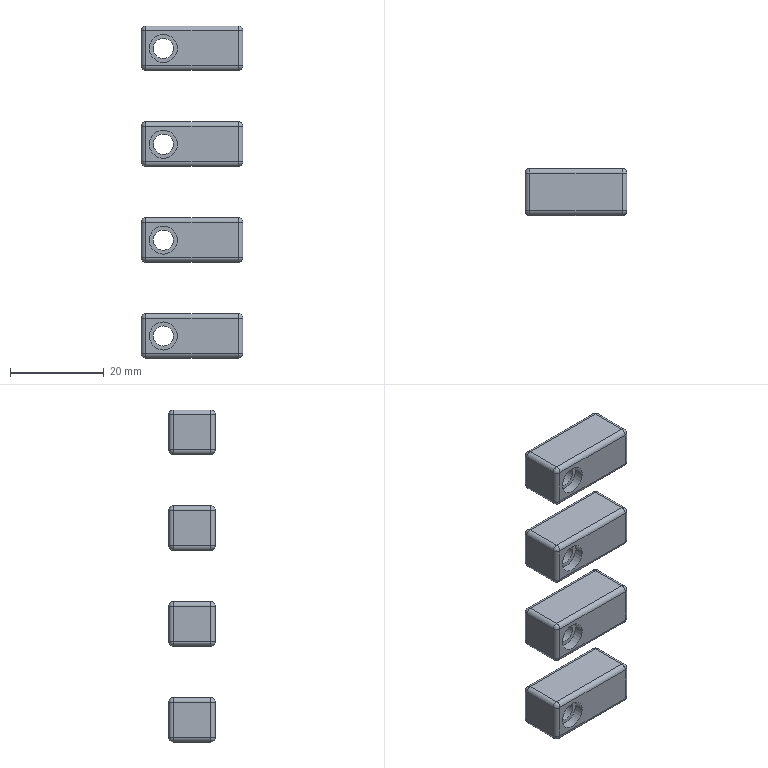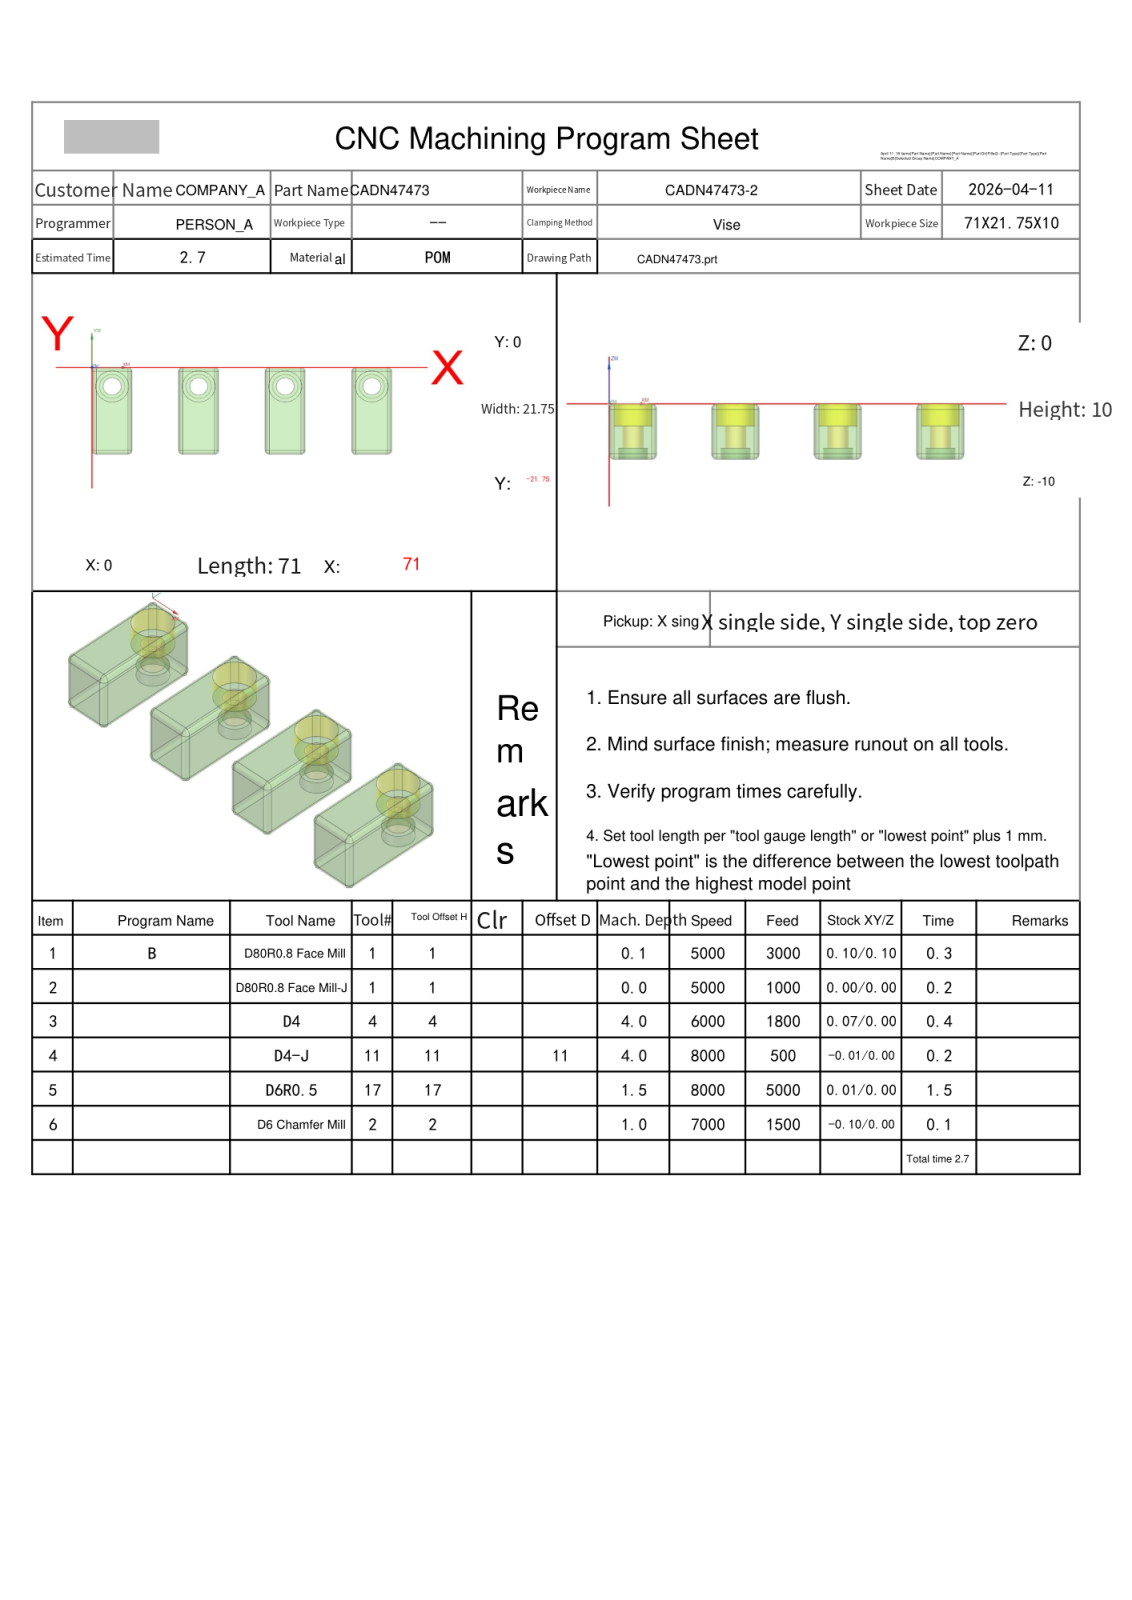NC program | NX | posted by the shop | part box 21.75 x 10 x 71 mm
Lines 1 to 259 of 15118:
%
O0001
(Machine time: 3.82 MIN)
(===Total Tool:5===)
(T1=D80R0.8 Face Mill D=80.  R=0.8  D-  H01 Z=0.    )
(T4=D4      D=4.   R=0.   D-  H04 Z=-4.   )
(T11=D4-J   D=4.   R=0.   D11 H11 Z=-4.   )
(T17=D6R0.5 D=6.   R=0.5  D-  H17 Z=-1.5  )
(T2=D6 Chamfer Mill   D=6.   R=0.   D-  H02 Z=-1.   )
G80 G90 G17 G49 G40
G91 G28 Z0
M01
N1 T01 M06
(D80R0.8 Face Mill  D=80. R=0.8 H=01 ce=0.10 di=0.10)
G00 G90 G54 X-52.097 Y-10.875 M03 S5000
G43 H01 Z20.
M08
Z3.525
G01 Z1.525 F3000.
X-40.097
X111.097
X123.097
Z3.525
G00 X-52.097
Z3.05
G01 Z1.05
X-40.097
X111.097
X123.097
Z3.05
G00 X-52.097
Z2.575
G01 Z.575
X-40.097
X111.097
X123.097
Z2.575
G00 X-52.097
Z2.1
G01 Z.1
X-40.097
X111.097
X123.097
Z2.1
G00 Z20.
G91 G28 Z0.0
M05
M09
G91 G28 Z0.0
M01
N2 T01 M06
(D80R0.8 Face Mill-J  D=80. R=0.8 H=01 ce=0.00 di=0.00)
G00 G90 G54 X-51.999 Y-10.875 M03 S5000
G43 H01 Z20.
M08
Z2.
G01 Z0.0 F1000.
X-39.999
X110.999
X122.999
Z2.
G00 Z20.
G91 G28 Z0.0
M05
M09
G91 G28 Z0.0
M01
N3 T04 M06
(D4  D=4. R=0. H=04 ce=0.07 di=0.00)
G00 G90 G54 X66.296 Y-4.75 M03 S6000
G43 H04 Z20.
M08
Z.3
G03 X65.381 Y-5.665 I0.0 J-.915 F1800.
X66.296 Y-6.58 I.915 J0.0
X66.296 Y-6.58 Z-.05 I0.0 J1.83
X66.296 Y-6.58 Z-.4 I0.0 J1.83
X66.296 Y-6.58 Z-.75 I0.0 J1.83
X66.296 Y-6.58 Z-1.1 I0.0 J1.83
X66.296 Y-6.58 Z-1.45 I0.0 J1.83
X66.296 Y-6.58 Z-1.8 I0.0 J1.83
X66.296 Y-6.58 Z-2.15 I0.0 J1.83
X66.296 Y-6.58 Z-2.5 I0.0 J1.83
X66.296 Y-6.58 Z-2.85 I0.0 J1.83
X66.296 Y-6.58 Z-3.2 I0.0 J1.83
X66.296 Y-6.58 Z-3.55 I0.0 J1.83
X66.296 Y-6.58 Z-3.9 I0.0 J1.83
X68.08 Y-4.343 Z-4. I0.0 J1.83
X66.296 Y-2.92 I-1.784 J-.407
X64.466 Y-4.75 I0.0 J-1.83
X66.296 Y-6.58 I1.83 J0.0
X68.126 Y-4.75 I0.0 J1.83
X68.08 Y-4.343 I-1.83 J0.0
X67.188 Y-3.631 I-.892 J-.204
X66.273 Y-4.546 I0.0 J-.915
X66.296 Y-4.75 I.915 J0.0
G00 Z20.
X45.796
Z.3
G03 X44.881 Y-5.665 I0.0 J-.915
X45.796 Y-6.58 I.915 J0.0
X45.796 Y-6.58 Z-.05 I0.0 J1.83
X45.796 Y-6.58 Z-.4 I0.0 J1.83
X45.796 Y-6.58 Z-.75 I0.0 J1.83
X45.796 Y-6.58 Z-1.1 I0.0 J1.83
X45.796 Y-6.58 Z-1.45 I0.0 J1.83
X45.796 Y-6.58 Z-1.8 I0.0 J1.83
X45.796 Y-6.58 Z-2.15 I0.0 J1.83
X45.796 Y-6.58 Z-2.5 I0.0 J1.83
X45.796 Y-6.58 Z-2.85 I0.0 J1.83
X45.796 Y-6.58 Z-3.2 I0.0 J1.83
X45.796 Y-6.58 Z-3.55 I0.0 J1.83
X45.796 Y-6.58 Z-3.9 I0.0 J1.83
X47.58 Y-4.343 Z-4. I0.0 J1.83
X45.796 Y-2.92 I-1.784 J-.407
X43.966 Y-4.75 I0.0 J-1.83
X45.796 Y-6.58 I1.83 J0.0
X47.626 Y-4.75 I0.0 J1.83
X47.58 Y-4.343 I-1.83 J0.0
X46.688 Y-3.631 I-.892 J-.204
X45.773 Y-4.546 I0.0 J-.915
X45.796 Y-4.75 I.915 J0.0
G00 Z20.
X25.296
Z.3
G03 X24.381 Y-5.665 I0.0 J-.915
X25.296 Y-6.58 I.915 J0.0
X25.296 Y-6.58 Z-.05 I0.0 J1.83
X25.296 Y-6.58 Z-.4 I0.0 J1.83
X25.296 Y-6.58 Z-.75 I0.0 J1.83
X25.296 Y-6.58 Z-1.1 I0.0 J1.83
X25.296 Y-6.58 Z-1.45 I0.0 J1.83
X25.296 Y-6.58 Z-1.8 I0.0 J1.83
X25.296 Y-6.58 Z-2.15 I0.0 J1.83
X25.296 Y-6.58 Z-2.5 I0.0 J1.83
X25.296 Y-6.58 Z-2.85 I0.0 J1.83
X25.296 Y-6.58 Z-3.2 I0.0 J1.83
X25.296 Y-6.58 Z-3.55 I0.0 J1.83
X25.296 Y-6.58 Z-3.9 I0.0 J1.83
X27.08 Y-4.343 Z-4. I0.0 J1.83
X25.296 Y-2.92 I-1.784 J-.407
X23.466 Y-4.75 I0.0 J-1.83
X25.296 Y-6.58 I1.83 J0.0
X27.126 Y-4.75 I0.0 J1.83
X27.08 Y-4.343 I-1.83 J0.0
X26.188 Y-3.631 I-.892 J-.204
X25.273 Y-4.546 I0.0 J-.915
X25.296 Y-4.75 I.915 J0.0
G00 Z20.
X4.796
Z.3
G03 X3.881 Y-5.665 I0.0 J-.915
X4.796 Y-6.58 I.915 J0.0
X4.796 Y-6.58 Z-.05 I0.0 J1.83
X4.796 Y-6.58 Z-.4 I0.0 J1.83
X4.796 Y-6.58 Z-.75 I0.0 J1.83
X4.796 Y-6.58 Z-1.1 I0.0 J1.83
X4.796 Y-6.58 Z-1.45 I0.0 J1.83
X4.796 Y-6.58 Z-1.8 I0.0 J1.83
X4.796 Y-6.58 Z-2.15 I0.0 J1.83
X4.796 Y-6.58 Z-2.5 I0.0 J1.83
X4.796 Y-6.58 Z-2.85 I0.0 J1.83
X4.796 Y-6.58 Z-3.2 I0.0 J1.83
X4.796 Y-6.58 Z-3.55 I0.0 J1.83
X4.796 Y-6.58 Z-3.9 I0.0 J1.83
X6.58 Y-4.343 Z-4. I0.0 J1.83
X4.796 Y-2.92 I-1.784 J-.407
X2.966 Y-4.75 I0.0 J-1.83
X4.796 Y-6.58 I1.83 J0.0
X6.626 Y-4.75 I0.0 J1.83
X6.58 Y-4.343 I-1.83 J0.0
X5.688 Y-3.631 I-.892 J-.204
X4.773 Y-4.546 I0.0 J-.915
X4.796 Y-4.75 I.915 J0.0
G00 Z20.
G91 G28 Z0.0
M05
M09
G91 G28 Z0.0
M01
N4 T11 M06
(D4-J  D=4. R=0. H=11 ce=-0.01 di=0.00)
G00 G90 G54 X66.866 Y-5.55 M03 S8000
G43 H11 Z11.8
M08
Z-3.
G01 Z-4. F500.
G41 D11
X67.406
G03 X68.206 Y-4.75 I0.0 J.8
X66.296 Y-2.84 I-1.91 J0.0
X64.386 Y-4.75 I0.0 J-1.91
X66.296 Y-6.66 I1.91 J0.0
X68.206 Y-4.75 I0.0 J1.91
X68.164 Y-4.353 I-1.91 J0.0
X67.382 Y-3.719 I-.783 J-.166
G01 X67.216 Y-3.737
X66.883 Y-3.808
G40 X66.687 Y-3.849
Z-3.
G00 Z11.8
X46.596 Y-4.181
Z-3.
G01 Z-4.
G41 D11
Y-3.64
G03 X45.796 Y-2.84 I-.8 J0.0
X43.886 Y-4.75 I0.0 J-1.91
X45.796 Y-6.66 I1.91 J0.0
X47.706 Y-4.75 I0.0 J1.91
X45.796 Y-2.84 I-1.91 J0.0
X45.399 Y-2.882 I0.0 J-1.91
X44.765 Y-3.664 I.166 J-.783
G01 X44.783 Y-3.831
X44.854 Y-4.164
G40 X44.895 Y-4.359
Z-3.
G00 Z11.8
X26.096 Y-4.181
Z-3.
G01 Z-4.
G41 D11
Y-3.64
G03 X25.296 Y-2.84 I-.8 J0.0
X23.386 Y-4.75 I0.0 J-1.91
X25.296 Y-6.66 I1.91 J0.0
X27.206 Y-4.75 I0.0 J1.91
X25.296 Y-2.84 I-1.91 J0.0
X24.899 Y-2.882 I0.0 J-1.91
X24.265 Y-3.664 I.166 J-.783
G01 X24.283 Y-3.831
X24.354 Y-4.164
G40 X24.395 Y-4.359
Z-3.
G00 Z11.8
X5.596 Y-4.181
Z-3.
G01 Z-4.
G41 D11
Y-3.64
G03 X4.796 Y-2.84 I-.8 J0.0
X2.886 Y-4.75 I0.0 J-1.91
X4.796 Y-6.66 I1.91 J0.0
X6.706 Y-4.75 I0.0 J1.91
X4.796 Y-2.84 I-1.91 J0.0
X4.399 Y-2.882 I0.0 J-1.91
X3.765 Y-3.664 I.166 J-.783
G01 X3.783 Y-3.831
X3.854 Y-4.164
G40 X3.895 Y-4.359
Z-3.
G00 Z11.8
G91 G28 Z0.0
M05
M09
G91 G28 Z0.0
M01